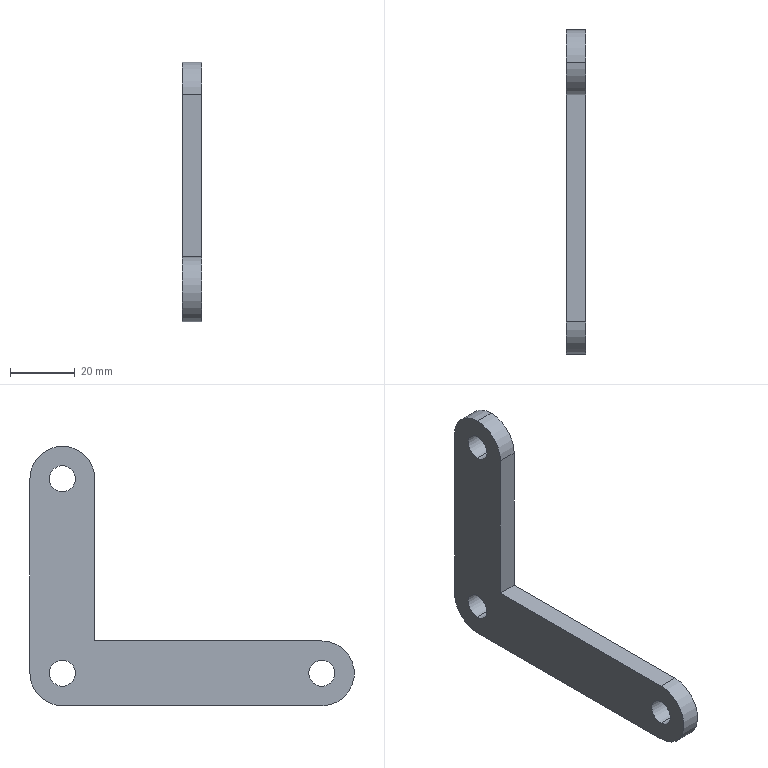Part | SolidWorks | features Extrusion 1 | 1 solid | 16 faces | box 6 x 100 x 80 mm | volume 17651 mm3 | cylinder 10 | plane 6 | commonest cylinder face diameters 8 x6 20 x4
STEP:
#1=CARTESIAN_POINT('',(6.,-80.,-56.));
#2=VERTEX_POINT('',#1);
#3=CARTESIAN_POINT('',(6.,-80.,-64.));
#4=VERTEX_POINT('',#3);
#5=CARTESIAN_POINT('',(6.,-80.,-60.));
#6=DIRECTION('',(1.,0.,0.));
#7=DIRECTION('',(0.,0.,-1.));
#8=AXIS2_PLACEMENT_3D('',#5,#6,#7);
#9=CIRCLE('',#8,4.);
#10=EDGE_CURVE('',#2,#4,#9,.T.);
#11=ORIENTED_EDGE('',*,*,#10,.T.);
#12=CARTESIAN_POINT('',(0.,-80.,-64.));
#13=VERTEX_POINT('',#12);
#14=CARTESIAN_POINT('',(6.,-80.,-64.));
#15=DIRECTION('',(-1.,0.,0.));
#16=VECTOR('',#15,1000.);
#17=LINE('',#14,#16);
#18=EDGE_CURVE('',#4,#13,#17,.T.);
#19=ORIENTED_EDGE('',*,*,#18,.T.);
#20=CARTESIAN_POINT('',(0.,-80.,-56.));
#21=VERTEX_POINT('',#20);
#22=CARTESIAN_POINT('',(0.,-80.,-60.));
#23=DIRECTION('',(1.,0.,0.));
#24=DIRECTION('',(0.,0.,-1.));
#25=AXIS2_PLACEMENT_3D('',#22,#23,#24);
#26=CIRCLE('',#25,4.);
#27=EDGE_CURVE('',#21,#13,#26,.T.);
#28=ORIENTED_EDGE('',*,*,#27,.F.);
#29=CARTESIAN_POINT('',(6.,-80.,-56.));
#30=DIRECTION('',(-1.,0.,0.));
#31=VECTOR('',#30,1000.);
#32=LINE('',#29,#31);
#33=EDGE_CURVE('',#2,#21,#32,.T.);
#34=ORIENTED_EDGE('',*,*,#33,.F.);
#35=EDGE_LOOP('',(#11,#19,#28,#34));
#36=FACE_OUTER_BOUND('',#35,.T.);
#37=CARTESIAN_POINT('',(6.,-80.,-60.));
#38=DIRECTION('',(-1.,0.,0.));
#39=DIRECTION('',(0.,0.,1.));
#40=AXIS2_PLACEMENT_3D('',#37,#38,#39);
#41=CYLINDRICAL_SURFACE('',#40,4.);
#42=ADVANCED_FACE('',(#36),#41,.F.);
#43=CARTESIAN_POINT('',(6.,0.,4.));
#44=VERTEX_POINT('',#43);
#45=CARTESIAN_POINT('',(6.,0.,-4.));
#46=VERTEX_POINT('',#45);
#47=CARTESIAN_POINT('',(6.,0.,0.));
#48=DIRECTION('',(1.,0.,0.));
#49=DIRECTION('',(0.,0.,-1.));
#50=AXIS2_PLACEMENT_3D('',#47,#48,#49);
#51=CIRCLE('',#50,4.);
#52=EDGE_CURVE('',#44,#46,#51,.T.);
#53=ORIENTED_EDGE('',*,*,#52,.T.);
#54=CARTESIAN_POINT('',(0.,0.,-4.));
#55=VERTEX_POINT('',#54);
#56=CARTESIAN_POINT('',(6.,0.,-4.));
#57=DIRECTION('',(-1.,0.,0.));
#58=VECTOR('',#57,1000.);
#59=LINE('',#56,#58);
#60=EDGE_CURVE('',#46,#55,#59,.T.);
#61=ORIENTED_EDGE('',*,*,#60,.T.);
#62=CARTESIAN_POINT('',(0.,0.,4.));
#63=VERTEX_POINT('',#62);
#64=CARTESIAN_POINT('',(0.,0.,0.));
#65=DIRECTION('',(1.,0.,0.));
#66=DIRECTION('',(0.,0.,-1.));
#67=AXIS2_PLACEMENT_3D('',#64,#65,#66);
#68=CIRCLE('',#67,4.);
#69=EDGE_CURVE('',#63,#55,#68,.T.);
#70=ORIENTED_EDGE('',*,*,#69,.F.);
#71=CARTESIAN_POINT('',(6.,0.,4.));
#72=DIRECTION('',(-1.,0.,0.));
#73=VECTOR('',#72,1000.);
#74=LINE('',#71,#73);
#75=EDGE_CURVE('',#44,#63,#74,.T.);
#76=ORIENTED_EDGE('',*,*,#75,.F.);
#77=EDGE_LOOP('',(#53,#61,#70,#76));
#78=FACE_OUTER_BOUND('',#77,.T.);
#79=CARTESIAN_POINT('',(6.,0.,0.));
#80=DIRECTION('',(-1.,0.,0.));
#81=DIRECTION('',(0.,0.,1.));
#82=AXIS2_PLACEMENT_3D('',#79,#80,#81);
#83=CYLINDRICAL_SURFACE('',#82,4.);
#84=ADVANCED_FACE('',(#78),#83,.F.);
#85=CARTESIAN_POINT('',(6.,0.,-56.));
#86=VERTEX_POINT('',#85);
#87=CARTESIAN_POINT('',(6.,0.,-64.));
#88=VERTEX_POINT('',#87);
#89=CARTESIAN_POINT('',(6.,0.,-60.));
#90=DIRECTION('',(1.,0.,0.));
#91=DIRECTION('',(0.,0.,-1.));
#92=AXIS2_PLACEMENT_3D('',#89,#90,#91);
#93=CIRCLE('',#92,4.);
#94=EDGE_CURVE('',#86,#88,#93,.T.);
#95=ORIENTED_EDGE('',*,*,#94,.T.);
#96=CARTESIAN_POINT('',(0.,0.,-64.));
#97=VERTEX_POINT('',#96);
#98=CARTESIAN_POINT('',(6.,0.,-64.));
#99=DIRECTION('',(-1.,0.,0.));
#100=VECTOR('',#99,1000.);
#101=LINE('',#98,#100);
#102=EDGE_CURVE('',#88,#97,#101,.T.);
#103=ORIENTED_EDGE('',*,*,#102,.T.);
#104=CARTESIAN_POINT('',(0.,0.,-56.));
#105=VERTEX_POINT('',#104);
#106=CARTESIAN_POINT('',(0.,0.,-60.));
#107=DIRECTION('',(1.,0.,0.));
#108=DIRECTION('',(0.,0.,-1.));
#109=AXIS2_PLACEMENT_3D('',#106,#107,#108);
#110=CIRCLE('',#109,4.);
#111=EDGE_CURVE('',#105,#97,#110,.T.);
#112=ORIENTED_EDGE('',*,*,#111,.F.);
#113=CARTESIAN_POINT('',(6.,0.,-56.));
#114=DIRECTION('',(-1.,0.,0.));
#115=VECTOR('',#114,1000.);
#116=LINE('',#113,#115);
#117=EDGE_CURVE('',#86,#105,#116,.T.);
#118=ORIENTED_EDGE('',*,*,#117,.F.);
#119=EDGE_LOOP('',(#95,#103,#112,#118));
#120=FACE_OUTER_BOUND('',#119,.T.);
#121=CARTESIAN_POINT('',(6.,0.,-60.));
#122=DIRECTION('',(-1.,0.,0.));
#123=DIRECTION('',(0.,0.,1.));
#124=AXIS2_PLACEMENT_3D('',#121,#122,#123);
#125=CYLINDRICAL_SURFACE('',#124,4.);
#126=ADVANCED_FACE('',(#120),#125,.F.);
#127=CARTESIAN_POINT('',(6.,0.,10.));
#128=VERTEX_POINT('',#127);
#129=CARTESIAN_POINT('',(6.,-10.,0.));
#130=VERTEX_POINT('',#129);
#131=CARTESIAN_POINT('',(6.,0.,0.));
#132=DIRECTION('',(1.,0.,0.));
#133=DIRECTION('',(0.,0.,-1.));
#134=AXIS2_PLACEMENT_3D('',#131,#132,#133);
#135=CIRCLE('',#134,10.);
#136=EDGE_CURVE('',#128,#130,#135,.T.);
#137=ORIENTED_EDGE('',*,*,#136,.F.);
#138=CARTESIAN_POINT('',(0.,0.,10.));
#139=VERTEX_POINT('',#138);
#140=CARTESIAN_POINT('',(6.,0.,10.));
#141=DIRECTION('',(-1.,0.,0.));
#142=VECTOR('',#141,1000.);
#143=LINE('',#140,#142);
#144=EDGE_CURVE('',#128,#139,#143,.T.);
#145=ORIENTED_EDGE('',*,*,#144,.T.);
#146=CARTESIAN_POINT('',(0.,-10.,0.));
#147=VERTEX_POINT('',#146);
#148=CARTESIAN_POINT('',(0.,0.,0.));
#149=DIRECTION('',(1.,0.,0.));
#150=DIRECTION('',(0.,0.,-1.));
#151=AXIS2_PLACEMENT_3D('',#148,#149,#150);
#152=CIRCLE('',#151,10.);
#153=EDGE_CURVE('',#139,#147,#152,.T.);
#154=ORIENTED_EDGE('',*,*,#153,.T.);
#155=CARTESIAN_POINT('',(6.,-10.,0.));
#156=DIRECTION('',(-1.,0.,0.));
#157=VECTOR('',#156,1000.);
#158=LINE('',#155,#157);
#159=EDGE_CURVE('',#130,#147,#158,.T.);
#160=ORIENTED_EDGE('',*,*,#159,.F.);
#161=EDGE_LOOP('',(#137,#145,#154,#160));
#162=FACE_OUTER_BOUND('',#161,.T.);
#163=CARTESIAN_POINT('',(6.,0.,0.));
#164=DIRECTION('',(-1.,0.,0.));
#165=DIRECTION('',(0.,0.,1.));
#166=AXIS2_PLACEMENT_3D('',#163,#164,#165);
#167=CYLINDRICAL_SURFACE('',#166,10.);
#168=ADVANCED_FACE('',(#162),#167,.T.);
#169=CARTESIAN_POINT('',(0.,0.,-70.));
#170=VERTEX_POINT('',#169);
#171=CARTESIAN_POINT('',(0.,-80.,-70.));
#172=VERTEX_POINT('',#171);
#173=CARTESIAN_POINT('',(0.,0.,-70.));
#174=DIRECTION('',(0.,-1.,0.));
#175=VECTOR('',#174,1000.);
#176=LINE('',#173,#175);
#177=EDGE_CURVE('',#170,#172,#176,.T.);
#178=ORIENTED_EDGE('',*,*,#177,.F.);
#179=CARTESIAN_POINT('',(6.,0.,-70.));
#180=VERTEX_POINT('',#179);
#181=CARTESIAN_POINT('',(6.,0.,-70.));
#182=DIRECTION('',(-1.,0.,0.));
#183=VECTOR('',#182,1000.);
#184=LINE('',#181,#183);
#185=EDGE_CURVE('',#180,#170,#184,.T.);
#186=ORIENTED_EDGE('',*,*,#185,.F.);
#187=CARTESIAN_POINT('',(6.,-80.,-70.));
#188=VERTEX_POINT('',#187);
#189=CARTESIAN_POINT('',(6.,0.,-70.));
#190=DIRECTION('',(0.,-1.,0.));
#191=VECTOR('',#190,1000.);
#192=LINE('',#189,#191);
#193=EDGE_CURVE('',#180,#188,#192,.T.);
#194=ORIENTED_EDGE('',*,*,#193,.T.);
#195=CARTESIAN_POINT('',(6.,-80.,-70.));
#196=DIRECTION('',(-1.,0.,0.));
#197=VECTOR('',#196,1000.);
#198=LINE('',#195,#197);
#199=EDGE_CURVE('',#188,#172,#198,.T.);
#200=ORIENTED_EDGE('',*,*,#199,.T.);
#201=EDGE_LOOP('',(#178,#186,#194,#200));
#202=FACE_OUTER_BOUND('',#201,.T.);
#203=CARTESIAN_POINT('',(6.,0.,-70.));
#204=DIRECTION('',(0.,0.,-1.));
#205=DIRECTION('',(-1.,0.,0.));
#206=AXIS2_PLACEMENT_3D('',#203,#204,#205);
#207=PLANE('',#206);
#208=ADVANCED_FACE('',(#202),#207,.T.);
#209=CARTESIAN_POINT('',(0.,10.,-60.));
#210=VERTEX_POINT('',#209);
#211=CARTESIAN_POINT('',(0.,0.,-60.));
#212=DIRECTION('',(1.,0.,0.));
#213=DIRECTION('',(0.,0.,-1.));
#214=AXIS2_PLACEMENT_3D('',#211,#212,#213);
#215=CIRCLE('',#214,10.);
#216=EDGE_CURVE('',#170,#210,#215,.T.);
#217=ORIENTED_EDGE('',*,*,#216,.T.);
#218=CARTESIAN_POINT('',(6.,10.,-60.));
#219=VERTEX_POINT('',#218);
#220=CARTESIAN_POINT('',(6.,10.,-60.));
#221=DIRECTION('',(-1.,0.,0.));
#222=VECTOR('',#221,1000.);
#223=LINE('',#220,#222);
#224=EDGE_CURVE('',#219,#210,#223,.T.);
#225=ORIENTED_EDGE('',*,*,#224,.F.);
#226=CARTESIAN_POINT('',(6.,0.,-60.));
#227=DIRECTION('',(1.,0.,0.));
#228=DIRECTION('',(0.,0.,-1.));
#229=AXIS2_PLACEMENT_3D('',#226,#227,#228);
#230=CIRCLE('',#229,10.);
#231=EDGE_CURVE('',#180,#219,#230,.T.);
#232=ORIENTED_EDGE('',*,*,#231,.F.);
#233=ORIENTED_EDGE('',*,*,#185,.T.);
#234=EDGE_LOOP('',(#217,#225,#232,#233));
#235=FACE_OUTER_BOUND('',#234,.T.);
#236=CARTESIAN_POINT('',(6.,0.,-60.));
#237=DIRECTION('',(-1.,0.,0.));
#238=DIRECTION('',(0.,0.,1.));
#239=AXIS2_PLACEMENT_3D('',#236,#237,#238);
#240=CYLINDRICAL_SURFACE('',#239,10.);
#241=ADVANCED_FACE('',(#235),#240,.T.);
#242=CARTESIAN_POINT('',(0.,10.,0.));
#243=VERTEX_POINT('',#242);
#244=CARTESIAN_POINT('',(0.,10.,0.));
#245=DIRECTION('',(0.,0.,-1.));
#246=VECTOR('',#245,1000.);
#247=LINE('',#244,#246);
#248=EDGE_CURVE('',#243,#210,#247,.T.);
#249=ORIENTED_EDGE('',*,*,#248,.F.);
#250=CARTESIAN_POINT('',(6.,10.,0.));
#251=VERTEX_POINT('',#250);
#252=CARTESIAN_POINT('',(6.,10.,0.));
#253=DIRECTION('',(-1.,0.,0.));
#254=VECTOR('',#253,1000.);
#255=LINE('',#252,#254);
#256=EDGE_CURVE('',#251,#243,#255,.T.);
#257=ORIENTED_EDGE('',*,*,#256,.F.);
#258=CARTESIAN_POINT('',(6.,10.,0.));
#259=DIRECTION('',(0.,0.,-1.));
#260=VECTOR('',#259,1000.);
#261=LINE('',#258,#260);
#262=EDGE_CURVE('',#251,#219,#261,.T.);
#263=ORIENTED_EDGE('',*,*,#262,.T.);
#264=ORIENTED_EDGE('',*,*,#224,.T.);
#265=EDGE_LOOP('',(#249,#257,#263,#264));
#266=FACE_OUTER_BOUND('',#265,.T.);
#267=CARTESIAN_POINT('',(6.,10.,0.));
#268=DIRECTION('',(0.,1.,0.));
#269=DIRECTION('',(0.,0.,1.));
#270=AXIS2_PLACEMENT_3D('',#267,#268,#269);
#271=PLANE('',#270);
#272=ADVANCED_FACE('',(#266),#271,.T.);
#273=ORIENTED_EDGE('',*,*,#144,.F.);
#274=CARTESIAN_POINT('',(6.,0.,0.));
#275=DIRECTION('',(1.,0.,0.));
#276=DIRECTION('',(0.,0.,-1.));
#277=AXIS2_PLACEMENT_3D('',#274,#275,#276);
#278=CIRCLE('',#277,10.);
#279=EDGE_CURVE('',#251,#128,#278,.T.);
#280=ORIENTED_EDGE('',*,*,#279,.F.);
#281=ORIENTED_EDGE('',*,*,#256,.T.);
#282=CARTESIAN_POINT('',(0.,0.,0.));
#283=DIRECTION('',(1.,0.,0.));
#284=DIRECTION('',(0.,0.,-1.));
#285=AXIS2_PLACEMENT_3D('',#282,#283,#284);
#286=CIRCLE('',#285,10.);
#287=EDGE_CURVE('',#243,#139,#286,.T.);
#288=ORIENTED_EDGE('',*,*,#287,.T.);
#289=EDGE_LOOP('',(#273,#280,#281,#288));
#290=FACE_OUTER_BOUND('',#289,.T.);
#291=CARTESIAN_POINT('',(6.,0.,0.));
#292=DIRECTION('',(-1.,0.,0.));
#293=DIRECTION('',(0.,0.,1.));
#294=AXIS2_PLACEMENT_3D('',#291,#292,#293);
#295=CYLINDRICAL_SURFACE('',#294,10.);
#296=ADVANCED_FACE('',(#290),#295,.T.);
#297=CARTESIAN_POINT('',(0.,-10.,-50.));
#298=VERTEX_POINT('',#297);
#299=CARTESIAN_POINT('',(0.,-10.,0.));
#300=DIRECTION('',(0.,0.,-1.));
#301=VECTOR('',#300,1000.);
#302=LINE('',#299,#301);
#303=EDGE_CURVE('',#147,#298,#302,.T.);
#304=ORIENTED_EDGE('',*,*,#303,.T.);
#305=CARTESIAN_POINT('',(6.,-10.,-50.));
#306=VERTEX_POINT('',#305);
#307=CARTESIAN_POINT('',(6.,-10.,-50.));
#308=DIRECTION('',(-1.,0.,0.));
#309=VECTOR('',#308,1000.);
#310=LINE('',#307,#309);
#311=EDGE_CURVE('',#306,#298,#310,.T.);
#312=ORIENTED_EDGE('',*,*,#311,.F.);
#313=CARTESIAN_POINT('',(6.,-10.,0.));
#314=DIRECTION('',(0.,0.,-1.));
#315=VECTOR('',#314,1000.);
#316=LINE('',#313,#315);
#317=EDGE_CURVE('',#130,#306,#316,.T.);
#318=ORIENTED_EDGE('',*,*,#317,.F.);
#319=ORIENTED_EDGE('',*,*,#159,.T.);
#320=EDGE_LOOP('',(#304,#312,#318,#319));
#321=FACE_OUTER_BOUND('',#320,.T.);
#322=CARTESIAN_POINT('',(6.,-10.,0.));
#323=DIRECTION('',(0.,1.,0.));
#324=DIRECTION('',(0.,0.,1.));
#325=AXIS2_PLACEMENT_3D('',#322,#323,#324);
#326=PLANE('',#325);
#327=ADVANCED_FACE('',(#321),#326,.F.);
#328=CARTESIAN_POINT('',(0.,-80.,-50.));
#329=VERTEX_POINT('',#328);
#330=CARTESIAN_POINT('',(0.,0.,-50.));
#331=DIRECTION('',(0.,-1.,0.));
#332=VECTOR('',#331,1000.);
#333=LINE('',#330,#332);
#334=EDGE_CURVE('',#298,#329,#333,.T.);
#335=ORIENTED_EDGE('',*,*,#334,.T.);
#336=CARTESIAN_POINT('',(6.,-80.,-50.));
#337=VERTEX_POINT('',#336);
#338=CARTESIAN_POINT('',(6.,-80.,-50.));
#339=DIRECTION('',(-1.,0.,0.));
#340=VECTOR('',#339,1000.);
#341=LINE('',#338,#340);
#342=EDGE_CURVE('',#337,#329,#341,.T.);
#343=ORIENTED_EDGE('',*,*,#342,.F.);
#344=CARTESIAN_POINT('',(6.,0.,-50.));
#345=DIRECTION('',(0.,-1.,0.));
#346=VECTOR('',#345,1000.);
#347=LINE('',#344,#346);
#348=EDGE_CURVE('',#306,#337,#347,.T.);
#349=ORIENTED_EDGE('',*,*,#348,.F.);
#350=ORIENTED_EDGE('',*,*,#311,.T.);
#351=EDGE_LOOP('',(#335,#343,#349,#350));
#352=FACE_OUTER_BOUND('',#351,.T.);
#353=CARTESIAN_POINT('',(6.,0.,-50.));
#354=DIRECTION('',(0.,0.,-1.));
#355=DIRECTION('',(0.,1.,0.));
#356=AXIS2_PLACEMENT_3D('',#353,#354,#355);
#357=PLANE('',#356);
#358=ADVANCED_FACE('',(#352),#357,.F.);
#359=ORIENTED_EDGE('',*,*,#102,.F.);
#360=CARTESIAN_POINT('',(6.,0.,-60.));
#361=DIRECTION('',(1.,0.,0.));
#362=DIRECTION('',(0.,0.,-1.));
#363=AXIS2_PLACEMENT_3D('',#360,#361,#362);
#364=CIRCLE('',#363,4.);
#365=EDGE_CURVE('',#88,#86,#364,.T.);
#366=ORIENTED_EDGE('',*,*,#365,.T.);
#367=ORIENTED_EDGE('',*,*,#117,.T.);
#368=CARTESIAN_POINT('',(0.,0.,-60.));
#369=DIRECTION('',(1.,0.,0.));
#370=DIRECTION('',(0.,0.,-1.));
#371=AXIS2_PLACEMENT_3D('',#368,#369,#370);
#372=CIRCLE('',#371,4.);
#373=EDGE_CURVE('',#97,#105,#372,.T.);
#374=ORIENTED_EDGE('',*,*,#373,.F.);
#375=EDGE_LOOP('',(#359,#366,#367,#374));
#376=FACE_OUTER_BOUND('',#375,.T.);
#377=CARTESIAN_POINT('',(6.,0.,-60.));
#378=DIRECTION('',(-1.,0.,0.));
#379=DIRECTION('',(0.,0.,1.));
#380=AXIS2_PLACEMENT_3D('',#377,#378,#379);
#381=CYLINDRICAL_SURFACE('',#380,4.);
#382=ADVANCED_FACE('',(#376),#381,.F.);
#383=ORIENTED_EDGE('',*,*,#60,.F.);
#384=CARTESIAN_POINT('',(6.,0.,0.));
#385=DIRECTION('',(1.,0.,0.));
#386=DIRECTION('',(0.,0.,-1.));
#387=AXIS2_PLACEMENT_3D('',#384,#385,#386);
#388=CIRCLE('',#387,4.);
#389=EDGE_CURVE('',#46,#44,#388,.T.);
#390=ORIENTED_EDGE('',*,*,#389,.T.);
#391=ORIENTED_EDGE('',*,*,#75,.T.);
#392=CARTESIAN_POINT('',(0.,0.,0.));
#393=DIRECTION('',(1.,0.,0.));
#394=DIRECTION('',(0.,0.,-1.));
#395=AXIS2_PLACEMENT_3D('',#392,#393,#394);
#396=CIRCLE('',#395,4.);
#397=EDGE_CURVE('',#55,#63,#396,.T.);
#398=ORIENTED_EDGE('',*,*,#397,.F.);
#399=EDGE_LOOP('',(#383,#390,#391,#398));
#400=FACE_OUTER_BOUND('',#399,.T.);
#401=CARTESIAN_POINT('',(6.,0.,0.));
#402=DIRECTION('',(-1.,0.,0.));
#403=DIRECTION('',(0.,0.,1.));
#404=AXIS2_PLACEMENT_3D('',#401,#402,#403);
#405=CYLINDRICAL_SURFACE('',#404,4.);
#406=ADVANCED_FACE('',(#400),#405,.F.);
#407=CARTESIAN_POINT('',(0.,-80.,-60.));
#408=DIRECTION('',(1.,0.,0.));
#409=DIRECTION('',(0.,0.,-1.));
#410=AXIS2_PLACEMENT_3D('',#407,#408,#409);
#411=CIRCLE('',#410,10.);
#412=EDGE_CURVE('',#329,#172,#411,.T.);
#413=ORIENTED_EDGE('',*,*,#412,.T.);
#414=ORIENTED_EDGE('',*,*,#199,.F.);
#415=CARTESIAN_POINT('',(6.,-80.,-60.));
#416=DIRECTION('',(1.,0.,0.));
#417=DIRECTION('',(0.,0.,-1.));
#418=AXIS2_PLACEMENT_3D('',#415,#416,#417);
#419=CIRCLE('',#418,10.);
#420=EDGE_CURVE('',#337,#188,#419,.T.);
#421=ORIENTED_EDGE('',*,*,#420,.F.);
#422=ORIENTED_EDGE('',*,*,#342,.T.);
#423=EDGE_LOOP('',(#413,#414,#421,#422));
#424=FACE_OUTER_BOUND('',#423,.T.);
#425=CARTESIAN_POINT('',(6.,-80.,-60.));
#426=DIRECTION('',(-1.,0.,0.));
#427=DIRECTION('',(0.,0.,1.));
#428=AXIS2_PLACEMENT_3D('',#425,#426,#427);
#429=CYLINDRICAL_SURFACE('',#428,10.);
#430=ADVANCED_FACE('',(#424),#429,.T.);
#431=ORIENTED_EDGE('',*,*,#18,.F.);
#432=CARTESIAN_POINT('',(6.,-80.,-60.));
#433=DIRECTION('',(1.,0.,0.));
#434=DIRECTION('',(0.,0.,-1.));
#435=AXIS2_PLACEMENT_3D('',#432,#433,#434);
#436=CIRCLE('',#435,4.);
#437=EDGE_CURVE('',#4,#2,#436,.T.);
#438=ORIENTED_EDGE('',*,*,#437,.T.);
#439=ORIENTED_EDGE('',*,*,#33,.T.);
#440=CARTESIAN_POINT('',(0.,-80.,-60.));
#441=DIRECTION('',(1.,0.,0.));
#442=DIRECTION('',(0.,0.,-1.));
#443=AXIS2_PLACEMENT_3D('',#440,#441,#442);
#444=CIRCLE('',#443,4.);
#445=EDGE_CURVE('',#13,#21,#444,.T.);
#446=ORIENTED_EDGE('',*,*,#445,.F.);
#447=EDGE_LOOP('',(#431,#438,#439,#446));
#448=FACE_OUTER_BOUND('',#447,.T.);
#449=CARTESIAN_POINT('',(6.,-80.,-60.));
#450=DIRECTION('',(-1.,0.,0.));
#451=DIRECTION('',(0.,0.,1.));
#452=AXIS2_PLACEMENT_3D('',#449,#450,#451);
#453=CYLINDRICAL_SURFACE('',#452,4.);
#454=ADVANCED_FACE('',(#448),#453,.F.);
#455=ORIENTED_EDGE('',*,*,#193,.F.);
#456=ORIENTED_EDGE('',*,*,#231,.T.);
#457=ORIENTED_EDGE('',*,*,#262,.F.);
#458=ORIENTED_EDGE('',*,*,#279,.T.);
#459=ORIENTED_EDGE('',*,*,#136,.T.);
#460=ORIENTED_EDGE('',*,*,#317,.T.);
#461=ORIENTED_EDGE('',*,*,#348,.T.);
#462=ORIENTED_EDGE('',*,*,#420,.T.);
#463=EDGE_LOOP('',(#455,#456,#457,#458,#459,#460,#461,#462));
#464=FACE_OUTER_BOUND('',#463,.T.);
#465=ORIENTED_EDGE('',*,*,#52,.F.);
#466=ORIENTED_EDGE('',*,*,#389,.F.);
#467=EDGE_LOOP('',(#465,#466));
#468=FACE_BOUND('',#467,.T.);
#469=ORIENTED_EDGE('',*,*,#94,.F.);
#470=ORIENTED_EDGE('',*,*,#365,.F.);
#471=EDGE_LOOP('',(#469,#470));
#472=FACE_BOUND('',#471,.T.);
#473=ORIENTED_EDGE('',*,*,#10,.F.);
#474=ORIENTED_EDGE('',*,*,#437,.F.);
#475=EDGE_LOOP('',(#473,#474));
#476=FACE_BOUND('',#475,.T.);
#477=CARTESIAN_POINT('',(6.,0.,0.));
#478=DIRECTION('',(1.,0.,0.));
#479=DIRECTION('',(0.,0.,-1.));
#480=AXIS2_PLACEMENT_3D('',#477,#478,#479);
#481=PLANE('',#480);
#482=ADVANCED_FACE('',(#464,#468,#472,#476),#481,.T.);
#483=ORIENTED_EDGE('',*,*,#177,.T.);
#484=ORIENTED_EDGE('',*,*,#412,.F.);
#485=ORIENTED_EDGE('',*,*,#334,.F.);
#486=ORIENTED_EDGE('',*,*,#303,.F.);
#487=ORIENTED_EDGE('',*,*,#153,.F.);
#488=ORIENTED_EDGE('',*,*,#287,.F.);
#489=ORIENTED_EDGE('',*,*,#248,.T.);
#490=ORIENTED_EDGE('',*,*,#216,.F.);
#491=EDGE_LOOP('',(#483,#484,#485,#486,#487,#488,#489,#490));
#492=FACE_OUTER_BOUND('',#491,.T.);
#493=ORIENTED_EDGE('',*,*,#69,.T.);
#494=ORIENTED_EDGE('',*,*,#397,.T.);
#495=EDGE_LOOP('',(#493,#494));
#496=FACE_BOUND('',#495,.T.);
#497=ORIENTED_EDGE('',*,*,#111,.T.);
#498=ORIENTED_EDGE('',*,*,#373,.T.);
#499=EDGE_LOOP('',(#497,#498));
#500=FACE_BOUND('',#499,.T.);
#501=ORIENTED_EDGE('',*,*,#27,.T.);
#502=ORIENTED_EDGE('',*,*,#445,.T.);
#503=EDGE_LOOP('',(#501,#502));
#504=FACE_BOUND('',#503,.T.);
#505=CARTESIAN_POINT('',(0.,0.,0.));
#506=DIRECTION('',(1.,0.,0.));
#507=DIRECTION('',(0.,0.,-1.));
#508=AXIS2_PLACEMENT_3D('',#505,#506,#507);
#509=PLANE('',#508);
#510=ADVANCED_FACE('',(#492,#496,#500,#504),#509,.F.);
#511=CLOSED_SHELL('',(#42,#84,#126,#168,#208,#241,#272,#296,#327,#358,#382,#406,#430,#454,#482,#510));
#512=MANIFOLD_SOLID_BREP('',#511);
#513=CARTESIAN_POINT('',(0.,0.,0.));
#514=DIRECTION('',(0.,0.,1.));
#515=DIRECTION('',(1.,0.,0.));
#516=AXIS2_PLACEMENT_3D('',#513,#514,#515);
#517=(LENGTH_UNIT()NAMED_UNIT(*)SI_UNIT(.MILLI.,.METRE.));
#518=UNCERTAINTY_MEASURE_WITH_UNIT(LENGTH_MEASURE(0.00001),#517,'','');
#519=(NAMED_UNIT(*)PLANE_ANGLE_UNIT()SI_UNIT($,.RADIAN.));
#520=(NAMED_UNIT(*)SI_UNIT($,.STERADIAN.)SOLID_ANGLE_UNIT());
#521=(GEOMETRIC_REPRESENTATION_CONTEXT(3)GLOBAL_UNCERTAINTY_ASSIGNED_CONTEXT((#518))GLOBAL_UNIT_ASSIGNED_CONTEXT((#517,#519,#520))REPRESENTATION_CONTEXT('',''));
#522=ADVANCED_BREP_SHAPE_REPRESENTATION('',(#512,#516),#521);